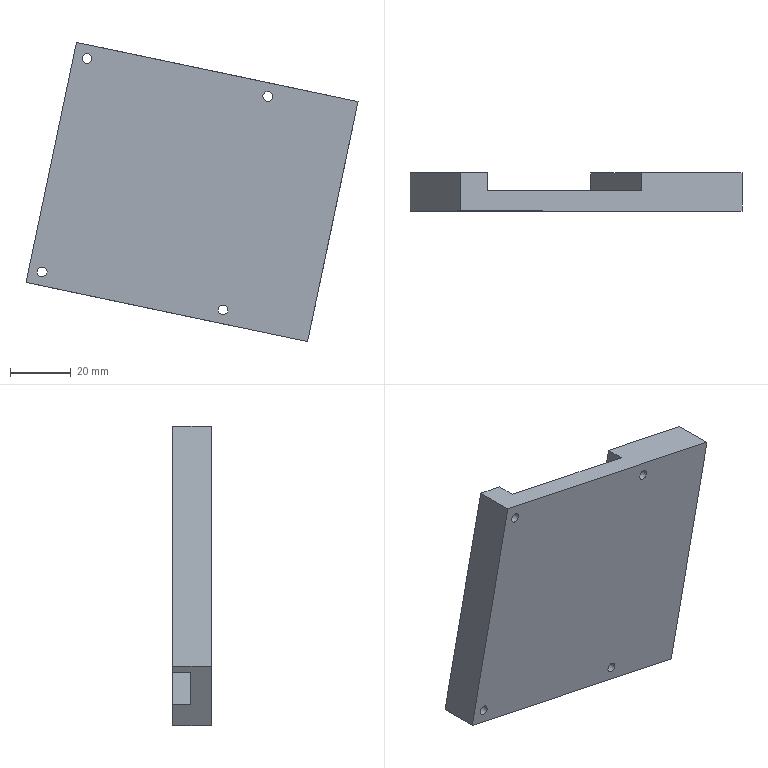Part | STEP file | 2_ESTAGIO_010 | 1 solid | 18 faces | box 109.627 x 12.7 x 98.805 mm | volume 71258 mm3 | plane 10 | cylinder 6 | cone 2 | commonest cylinder face diameters 3.242 x4 4.917 x2
STEP:
#1=CARTESIAN_POINT('',(0.,0.,0.));
#2=DIRECTION('',(0.,0.,1.));
#3=DIRECTION('',(1.,0.,0.));
#4=AXIS2_PLACEMENT_3D('',#1,#2,#3);
#5=CARTESIAN_POINT('',(428.339,-542.821,373.692));
#6=VERTEX_POINT('',#5);
#7=CARTESIAN_POINT('',(427.895,-544.,371.581));
#8=DIRECTION('',(0.9786,0.,-0.2056));
#9=DIRECTION('',(0.2056,0.,0.9786));
#10=AXIS2_PLACEMENT_3D('',#7,#8,#9);
#11=CIRCLE('',#10,2.458);
#12=CARTESIAN_POINT('',(427.071,-544.,371.754));
#13=DIRECTION('',(0.9786,0.,-0.2056));
#14=DIRECTION('',(0.1805,0.4794,0.8588));
#15=AXIS2_PLACEMENT_3D('',#12,#13,#14);
#16=CONICAL_SURFACE('',#15,1.,1.047);
#17=CARTESIAN_POINT('',(-5.783,0.8421));
#18=DIRECTION('',(1.,0.));
#19=VECTOR('',#18,1.);
#20=LINE('',#17,#19);
#21=(GEOMETRIC_REPRESENTATION_CONTEXT(2)PARAMETRIC_REPRESENTATION_CONTEXT()REPRESENTATION_CONTEXT('',''));
#22=DEFINITIONAL_REPRESENTATION('',(#20),#21);
#23=PCURVE('',#16,#22);
#24=CARTESIAN_POINT('',(447.37,-544.,367.488));
#25=DIRECTION('',(-0.9786,0.,0.2056));
#26=DIRECTION('',(0.1805,0.4794,0.8588));
#27=AXIS2_PLACEMENT_3D('',#24,#25,#26);
#28=CYLINDRICAL_SURFACE('',#27,2.458);
#29=CARTESIAN_POINT('',(12.066,19.9));
#30=DIRECTION('',(-1.,0.));
#31=VECTOR('',#30,1.);
#32=LINE('',#29,#31);
#33=(GEOMETRIC_REPRESENTATION_CONTEXT(2)PARAMETRIC_REPRESENTATION_CONTEXT()REPRESENTATION_CONTEXT('',''));
#34=DEFINITIONAL_REPRESENTATION('',(#32),#33);
#35=PCURVE('',#28,#34);
#36=SURFACE_CURVE('',#11,(#23,#35),.PCURVE_S1.);
#37=EDGE_CURVE('',#6,#6,#36,.T.);
#38=ORIENTED_EDGE('',*,*,#37,.F.);
#39=CARTESIAN_POINT('',(426.506,-544.,371.873));
#40=VERTEX_POINT('',#39);
#41=CARTESIAN_POINT('',(426.506,-544.,371.873));
#42=CARTESIAN_POINT('',(428.339,-542.821,373.692));
#43=B_SPLINE_CURVE_WITH_KNOTS('',1,(#41,#42),.UNSPECIFIED.,.F.,.F.,(2,2),(-1.155,1.684),.PIECEWISE_BEZIER_KNOTS.);
#44=CARTESIAN_POINT('',(0.,0.));
#45=DIRECTION('',(0.,1.));
#46=VECTOR('',#45,1.);
#47=LINE('',#44,#46);
#48=(GEOMETRIC_REPRESENTATION_CONTEXT(2)PARAMETRIC_REPRESENTATION_CONTEXT()REPRESENTATION_CONTEXT('',''));
#49=DEFINITIONAL_REPRESENTATION('',(#47),#48);
#50=PCURVE('',#16,#49);
#51=CARTESIAN_POINT('',(6.283,0.));
#52=DIRECTION('',(0.,1.));
#53=VECTOR('',#52,1.);
#54=LINE('',#51,#53);
#55=(GEOMETRIC_REPRESENTATION_CONTEXT(2)PARAMETRIC_REPRESENTATION_CONTEXT()REPRESENTATION_CONTEXT('',''));
#56=DEFINITIONAL_REPRESENTATION('',(#54),#55);
#57=PCURVE('',#16,#56);
#58=SEAM_CURVE('',#43,(#50,#57),.PCURVE_S1.);
#59=EDGE_CURVE('',#40,#6,#58,.T.);
#60=ORIENTED_EDGE('',*,*,#59,.F.);
#61=ORIENTED_EDGE('',*,*,#59,.T.);
#62=EDGE_LOOP('',(#38,#60,#61));
#63=FACE_BOUND('',#62,.F.);
#64=ADVANCED_FACE('',(#63),#16,.F.);
#65=CARTESIAN_POINT('',(443.355,-537.65,347.895));
#66=VERTEX_POINT('',#65);
#67=CARTESIAN_POINT('',(460.012,-537.65,427.164));
#68=VERTEX_POINT('',#67);
#69=CARTESIAN_POINT('',(443.355,-537.65,347.895));
#70=DIRECTION('',(0.2056,0.,0.9786));
#71=VECTOR('',#70,1.);
#72=LINE('',#69,#71);
#73=CARTESIAN_POINT('',(442.944,-550.35,345.938));
#74=DIRECTION('',(0.9786,0.,-0.2056));
#75=DIRECTION('',(-0.2056,0.,-0.9786));
#76=AXIS2_PLACEMENT_3D('',#73,#74,#75);
#77=PLANE('',#76);
#78=CARTESIAN_POINT('',(-2.,12.7));
#79=DIRECTION('',(-1.,0.));
#80=VECTOR('',#79,1.);
#81=LINE('',#78,#80);
#82=(GEOMETRIC_REPRESENTATION_CONTEXT(2)PARAMETRIC_REPRESENTATION_CONTEXT()REPRESENTATION_CONTEXT('',''));
#83=DEFINITIONAL_REPRESENTATION('',(#81),#82);
#84=PCURVE('',#77,#83);
#85=CARTESIAN_POINT('',(413.585,-537.65,352.107));
#86=DIRECTION('',(0.,1.,0.));
#87=DIRECTION('',(0.,0.,1.));
#88=AXIS2_PLACEMENT_3D('',#85,#86,#87);
#89=PLANE('',#88);
#90=CARTESIAN_POINT('',(-4.212,29.77));
#91=DIRECTION('',(0.9786,0.2056));
#92=VECTOR('',#91,1.);
#93=LINE('',#90,#92);
#94=(GEOMETRIC_REPRESENTATION_CONTEXT(2)PARAMETRIC_REPRESENTATION_CONTEXT()REPRESENTATION_CONTEXT('',''));
#95=DEFINITIONAL_REPRESENTATION('',(#93),#94);
#96=PCURVE('',#89,#95);
#97=SURFACE_CURVE('',#72,(#84,#96),.PCURVE_S1.);
#98=EDGE_CURVE('',#66,#68,#97,.T.);
#99=ORIENTED_EDGE('',*,*,#98,.T.);
#100=CARTESIAN_POINT('',(460.012,-550.35,427.164));
#101=VERTEX_POINT('',#100);
#102=CARTESIAN_POINT('',(460.012,-550.35,427.164));
#103=DIRECTION('',(0.,1.,0.));
#104=VECTOR('',#103,1.);
#105=LINE('',#102,#104);
#106=CARTESIAN_POINT('',(-83.,0.));
#107=DIRECTION('',(0.,1.));
#108=VECTOR('',#107,1.);
#109=LINE('',#106,#108);
#110=(GEOMETRIC_REPRESENTATION_CONTEXT(2)PARAMETRIC_REPRESENTATION_CONTEXT()REPRESENTATION_CONTEXT('',''));
#111=DEFINITIONAL_REPRESENTATION('',(#109),#110);
#112=PCURVE('',#77,#111);
#113=CARTESIAN_POINT('',(105.419,0.,501.676));
#114=DIRECTION('',(0.2056,0.,0.9786));
#115=DIRECTION('',(0.9786,0.,-0.2056));
#116=AXIS2_PLACEMENT_3D('',#113,#114,#115);
#117=PLANE('',#116);
#118=CARTESIAN_POINT('',(362.337,-550.35));
#119=DIRECTION('',(0.,1.));
#120=VECTOR('',#119,1.);
#121=LINE('',#118,#120);
#122=(GEOMETRIC_REPRESENTATION_CONTEXT(2)PARAMETRIC_REPRESENTATION_CONTEXT()REPRESENTATION_CONTEXT('',''));
#123=DEFINITIONAL_REPRESENTATION('',(#121),#122);
#124=PCURVE('',#117,#123);
#125=SURFACE_CURVE('',#105,(#112,#124),.PCURVE_S1.);
#126=EDGE_CURVE('',#101,#68,#125,.T.);
#127=ORIENTED_EDGE('',*,*,#126,.F.);
#128=CARTESIAN_POINT('',(443.355,-550.35,347.895));
#129=VERTEX_POINT('',#128);
#130=CARTESIAN_POINT('',(443.355,-550.35,347.895));
#131=DIRECTION('',(0.2056,0.,0.9786));
#132=VECTOR('',#131,1.);
#133=LINE('',#130,#132);
#134=CARTESIAN_POINT('',(-2.,0.));
#135=DIRECTION('',(-1.,0.));
#136=VECTOR('',#135,1.);
#137=LINE('',#134,#136);
#138=(GEOMETRIC_REPRESENTATION_CONTEXT(2)PARAMETRIC_REPRESENTATION_CONTEXT()REPRESENTATION_CONTEXT('',''));
#139=DEFINITIONAL_REPRESENTATION('',(#137),#138);
#140=PCURVE('',#77,#139);
#141=CARTESIAN_POINT('',(354.867,-550.35,364.446));
#142=DIRECTION('',(0.,-1.,0.));
#143=DIRECTION('',(0.,0.,-1.));
#144=AXIS2_PLACEMENT_3D('',#141,#142,#143);
#145=PLANE('',#144);
#146=CARTESIAN_POINT('',(16.551,88.488));
#147=DIRECTION('',(-0.9786,0.2056));
#148=VECTOR('',#147,1.);
#149=LINE('',#146,#148);
#150=(GEOMETRIC_REPRESENTATION_CONTEXT(2)PARAMETRIC_REPRESENTATION_CONTEXT()REPRESENTATION_CONTEXT('',''));
#151=DEFINITIONAL_REPRESENTATION('',(#149),#150);
#152=PCURVE('',#145,#151);
#153=SURFACE_CURVE('',#133,(#140,#152),.PCURVE_S1.);
#154=EDGE_CURVE('',#129,#101,#153,.T.);
#155=ORIENTED_EDGE('',*,*,#154,.F.);
#156=CARTESIAN_POINT('',(443.355,-550.35,347.895));
#157=DIRECTION('',(0.,1.,0.));
#158=VECTOR('',#157,1.);
#159=LINE('',#156,#158);
#160=CARTESIAN_POINT('',(-2.,0.));
#161=DIRECTION('',(0.,1.));
#162=VECTOR('',#161,1.);
#163=LINE('',#160,#162);
#164=(GEOMETRIC_REPRESENTATION_CONTEXT(2)PARAMETRIC_REPRESENTATION_CONTEXT()REPRESENTATION_CONTEXT('',''));
#165=DEFINITIONAL_REPRESENTATION('',(#163),#164);
#166=PCURVE('',#77,#165);
#167=CARTESIAN_POINT('',(88.762,0.,422.407));
#168=DIRECTION('',(0.2056,0.,0.9786));
#169=DIRECTION('',(0.9786,0.,-0.2056));
#170=AXIS2_PLACEMENT_3D('',#167,#168,#169);
#171=PLANE('',#170);
#172=CARTESIAN_POINT('',(362.337,-550.35));
#173=DIRECTION('',(0.,1.));
#174=VECTOR('',#173,1.);
#175=LINE('',#172,#174);
#176=(GEOMETRIC_REPRESENTATION_CONTEXT(2)PARAMETRIC_REPRESENTATION_CONTEXT()REPRESENTATION_CONTEXT('',''));
#177=DEFINITIONAL_REPRESENTATION('',(#175),#176);
#178=PCURVE('',#171,#177);
#179=SURFACE_CURVE('',#159,(#166,#178),.PCURVE_S1.);
#180=EDGE_CURVE('',#129,#66,#179,.T.);
#181=ORIENTED_EDGE('',*,*,#180,.T.);
#182=EDGE_LOOP('',(#99,#127,#155,#181));
#183=FACE_BOUND('',#182,.T.);
#184=CARTESIAN_POINT('',(447.912,-542.821,369.579));
#185=VERTEX_POINT('',#184);
#186=CARTESIAN_POINT('',(447.468,-544.,367.468));
#187=DIRECTION('',(0.9786,0.,-0.2056));
#188=DIRECTION('',(0.1805,0.4794,0.8588));
#189=AXIS2_PLACEMENT_3D('',#186,#187,#188);
#190=CIRCLE('',#189,2.458);
#191=CARTESIAN_POINT('',(-22.,6.35));
#192=DIRECTION('',(-0.8776,0.4794));
#193=AXIS2_PLACEMENT_2D('',#191,#192);
#194=CIRCLE('',#193,2.458);
#195=(GEOMETRIC_REPRESENTATION_CONTEXT(2)PARAMETRIC_REPRESENTATION_CONTEXT()REPRESENTATION_CONTEXT('',''));
#196=DEFINITIONAL_REPRESENTATION('',(#194),#195);
#197=PCURVE('',#77,#196);
#198=CARTESIAN_POINT('',(6.283,-0.1));
#199=DIRECTION('',(-1.,0.));
#200=VECTOR('',#199,1.);
#201=LINE('',#198,#200);
#202=(GEOMETRIC_REPRESENTATION_CONTEXT(2)PARAMETRIC_REPRESENTATION_CONTEXT()REPRESENTATION_CONTEXT('',''));
#203=DEFINITIONAL_REPRESENTATION('',(#201),#202);
#204=PCURVE('',#28,#203);
#205=SURFACE_CURVE('',#190,(#197,#204),.PCURVE_S1.);
#206=EDGE_CURVE('',#185,#185,#205,.T.);
#207=ORIENTED_EDGE('',*,*,#206,.F.);
#208=EDGE_LOOP('',(#207));
#209=FACE_BOUND('',#208,.T.);
#210=CARTESIAN_POINT('',(456.343,-542.821,409.703));
#211=VERTEX_POINT('',#210);
#212=CARTESIAN_POINT('',(455.899,-544.,407.592));
#213=DIRECTION('',(0.9786,0.,-0.2056));
#214=DIRECTION('',(0.1805,0.4794,0.8588));
#215=AXIS2_PLACEMENT_3D('',#212,#213,#214);
#216=CIRCLE('',#215,2.458);
#217=CARTESIAN_POINT('',(-63.,6.35));
#218=DIRECTION('',(-0.8776,0.4794));
#219=AXIS2_PLACEMENT_2D('',#217,#218);
#220=CIRCLE('',#219,2.458);
#221=(GEOMETRIC_REPRESENTATION_CONTEXT(2)PARAMETRIC_REPRESENTATION_CONTEXT()REPRESENTATION_CONTEXT('',''));
#222=DEFINITIONAL_REPRESENTATION('',(#220),#221);
#223=PCURVE('',#77,#222);
#224=CARTESIAN_POINT('',(455.801,-544.,407.612));
#225=DIRECTION('',(-0.9786,0.,0.2056));
#226=DIRECTION('',(0.1805,0.4794,0.8588));
#227=AXIS2_PLACEMENT_3D('',#224,#225,#226);
#228=CYLINDRICAL_SURFACE('',#227,2.458);
#229=CARTESIAN_POINT('',(6.283,-0.1));
#230=DIRECTION('',(-1.,0.));
#231=VECTOR('',#230,1.);
#232=LINE('',#229,#231);
#233=(GEOMETRIC_REPRESENTATION_CONTEXT(2)PARAMETRIC_REPRESENTATION_CONTEXT()REPRESENTATION_CONTEXT('',''));
#234=DEFINITIONAL_REPRESENTATION('',(#232),#233);
#235=PCURVE('',#228,#234);
#236=SURFACE_CURVE('',#216,(#223,#235),.PCURVE_S1.);
#237=EDGE_CURVE('',#211,#211,#236,.T.);
#238=ORIENTED_EDGE('',*,*,#237,.F.);
#239=EDGE_LOOP('',(#238));
#240=FACE_BOUND('',#239,.T.);
#241=ADVANCED_FACE('',(#183,#209,#240),#77,.T.);
#242=CARTESIAN_POINT('',(410.082,-537.65,354.887));
#243=VERTEX_POINT('',#242);
#244=CARTESIAN_POINT('',(410.082,-537.65,354.887));
#245=DIRECTION('',(0.9786,0.,-0.2056));
#246=VECTOR('',#245,1.);
#247=LINE('',#244,#246);
#248=CARTESIAN_POINT('',(2.78,-3.503));
#249=DIRECTION('',(-0.2056,0.9786));
#250=VECTOR('',#249,1.);
#251=LINE('',#248,#250);
#252=(GEOMETRIC_REPRESENTATION_CONTEXT(2)PARAMETRIC_REPRESENTATION_CONTEXT()REPRESENTATION_CONTEXT('',''));
#253=DEFINITIONAL_REPRESENTATION('',(#251),#252);
#254=PCURVE('',#89,#253);
#255=CARTESIAN_POINT('',(328.337,-537.65));
#256=DIRECTION('',(1.,0.));
#257=VECTOR('',#256,1.);
#258=LINE('',#255,#257);
#259=(GEOMETRIC_REPRESENTATION_CONTEXT(2)PARAMETRIC_REPRESENTATION_CONTEXT()REPRESENTATION_CONTEXT('',''));
#260=DEFINITIONAL_REPRESENTATION('',(#258),#259);
#261=PCURVE('',#171,#260);
#262=SURFACE_CURVE('',#247,(#254,#261),.PCURVE_S1.);
#263=EDGE_CURVE('',#243,#66,#262,.T.);
#264=ORIENTED_EDGE('',*,*,#263,.F.);
#265=CARTESIAN_POINT('',(426.739,-537.65,434.156));
#266=VERTEX_POINT('',#265);
#267=CARTESIAN_POINT('',(410.082,-537.65,354.887));
#268=DIRECTION('',(0.2056,0.,0.9786));
#269=VECTOR('',#268,1.);
#270=LINE('',#267,#269);
#271=CARTESIAN_POINT('',(2.78,-3.503));
#272=DIRECTION('',(0.9786,0.2056));
#273=VECTOR('',#272,1.);
#274=LINE('',#271,#273);
#275=(GEOMETRIC_REPRESENTATION_CONTEXT(2)PARAMETRIC_REPRESENTATION_CONTEXT()REPRESENTATION_CONTEXT('',''));
#276=DEFINITIONAL_REPRESENTATION('',(#274),#275);
#277=PCURVE('',#89,#276);
#278=CARTESIAN_POINT('',(409.67,-537.65,352.93));
#279=DIRECTION('',(-0.9786,0.,0.2056));
#280=DIRECTION('',(0.2056,0.,0.9786));
#281=AXIS2_PLACEMENT_3D('',#278,#279,#280);
#282=PLANE('',#281);
#283=CARTESIAN_POINT('',(2.,0.));
#284=DIRECTION('',(1.,0.));
#285=VECTOR('',#284,1.);
#286=LINE('',#283,#285);
#287=(GEOMETRIC_REPRESENTATION_CONTEXT(2)PARAMETRIC_REPRESENTATION_CONTEXT()REPRESENTATION_CONTEXT('',''));
#288=DEFINITIONAL_REPRESENTATION('',(#286),#287);
#289=PCURVE('',#282,#288);
#290=SURFACE_CURVE('',#270,(#277,#289),.PCURVE_S1.);
#291=EDGE_CURVE('',#243,#266,#290,.T.);
#292=ORIENTED_EDGE('',*,*,#291,.T.);
#293=CARTESIAN_POINT('',(426.739,-537.65,434.156));
#294=DIRECTION('',(0.9786,0.,-0.2056));
#295=VECTOR('',#294,1.);
#296=LINE('',#293,#295);
#297=CARTESIAN_POINT('',(82.049,13.154));
#298=DIRECTION('',(-0.2056,0.9786));
#299=VECTOR('',#298,1.);
#300=LINE('',#297,#299);
#301=(GEOMETRIC_REPRESENTATION_CONTEXT(2)PARAMETRIC_REPRESENTATION_CONTEXT()REPRESENTATION_CONTEXT('',''));
#302=DEFINITIONAL_REPRESENTATION('',(#300),#301);
#303=PCURVE('',#89,#302);
#304=CARTESIAN_POINT('',(328.337,-537.65));
#305=DIRECTION('',(1.,0.));
#306=VECTOR('',#305,1.);
#307=LINE('',#304,#306);
#308=(GEOMETRIC_REPRESENTATION_CONTEXT(2)PARAMETRIC_REPRESENTATION_CONTEXT()REPRESENTATION_CONTEXT('',''));
#309=DEFINITIONAL_REPRESENTATION('',(#307),#308);
#310=PCURVE('',#117,#309);
#311=SURFACE_CURVE('',#296,(#303,#310),.PCURVE_S1.);
#312=EDGE_CURVE('',#266,#68,#311,.T.);
#313=ORIENTED_EDGE('',*,*,#312,.T.);
#314=ORIENTED_EDGE('',*,*,#98,.F.);
#315=EDGE_LOOP('',(#264,#292,#313,#314));
#316=FACE_BOUND('',#315,.T.);
#317=CARTESIAN_POINT('',(428.795,-537.65,428.05));
#318=VERTEX_POINT('',#317);
#319=CARTESIAN_POINT('',(430.217,-537.65,428.827));
#320=DIRECTION('',(0.,1.,0.));
#321=DIRECTION('',(1.,0.,0.));
#322=AXIS2_PLACEMENT_3D('',#319,#320,#321);
#323=CIRCLE('',#322,1.621);
#324=CARTESIAN_POINT('',(76.719,16.632));
#325=DIRECTION('',(0.,1.));
#326=AXIS2_PLACEMENT_2D('',#324,#325);
#327=CIRCLE('',#326,1.621);
#328=(GEOMETRIC_REPRESENTATION_CONTEXT(2)PARAMETRIC_REPRESENTATION_CONTEXT()REPRESENTATION_CONTEXT('',''));
#329=DEFINITIONAL_REPRESENTATION('',(#327),#328);
#330=PCURVE('',#89,#329);
#331=CARTESIAN_POINT('',(430.217,-537.75,428.827));
#332=DIRECTION('',(0.,-1.,0.));
#333=DIRECTION('',(0.8776,0.,0.4794));
#334=AXIS2_PLACEMENT_3D('',#331,#332,#333);
#335=CYLINDRICAL_SURFACE('',#334,1.621);
#336=CARTESIAN_POINT('',(12.066,-0.1));
#337=DIRECTION('',(-1.,0.));
#338=VECTOR('',#337,1.);
#339=LINE('',#336,#338);
#340=(GEOMETRIC_REPRESENTATION_CONTEXT(2)PARAMETRIC_REPRESENTATION_CONTEXT()REPRESENTATION_CONTEXT('',''));
#341=DEFINITIONAL_REPRESENTATION('',(#339),#340);
#342=PCURVE('',#335,#341);
#343=SURFACE_CURVE('',#323,(#330,#342),.PCURVE_S1.);
#344=EDGE_CURVE('',#318,#318,#343,.T.);
#345=ORIENTED_EDGE('',*,*,#344,.F.);
#346=EDGE_LOOP('',(#345));
#347=FACE_BOUND('',#346,.T.);
#348=CARTESIAN_POINT('',(413.988,-537.65,357.588));
#349=VERTEX_POINT('',#348);
#350=CARTESIAN_POINT('',(415.411,-537.65,358.366));
#351=DIRECTION('',(0.,1.,0.));
#352=DIRECTION('',(1.,0.,0.));
#353=AXIS2_PLACEMENT_3D('',#350,#351,#352);
#354=CIRCLE('',#353,1.621);
#355=CARTESIAN_POINT('',(6.258,1.826));
#356=DIRECTION('',(0.,1.));
#357=AXIS2_PLACEMENT_2D('',#355,#356);
#358=CIRCLE('',#357,1.621);
#359=(GEOMETRIC_REPRESENTATION_CONTEXT(2)PARAMETRIC_REPRESENTATION_CONTEXT()REPRESENTATION_CONTEXT('',''));
#360=DEFINITIONAL_REPRESENTATION('',(#358),#359);
#361=PCURVE('',#89,#360);
#362=CARTESIAN_POINT('',(415.411,-537.75,358.366));
#363=DIRECTION('',(0.,-1.,0.));
#364=DIRECTION('',(0.8776,0.,0.4794));
#365=AXIS2_PLACEMENT_3D('',#362,#363,#364);
#366=CYLINDRICAL_SURFACE('',#365,1.621);
#367=CARTESIAN_POINT('',(12.066,-0.1));
#368=DIRECTION('',(-1.,0.));
#369=VECTOR('',#368,1.);
#370=LINE('',#367,#369);
#371=(GEOMETRIC_REPRESENTATION_CONTEXT(2)PARAMETRIC_REPRESENTATION_CONTEXT()REPRESENTATION_CONTEXT('',''));
#372=DEFINITIONAL_REPRESENTATION('',(#370),#371);
#373=PCURVE('',#366,#372);
#374=SURFACE_CURVE('',#354,(#361,#373),.PCURVE_S1.);
#375=EDGE_CURVE('',#349,#349,#374,.T.);
#376=ORIENTED_EDGE('',*,*,#375,.F.);
#377=EDGE_LOOP('',(#376));
#378=FACE_BOUND('',#377,.T.);
#379=ADVANCED_FACE('',(#316,#347,#378),#89,.T.);
#380=CARTESIAN_POINT('',(350.385,-550.35,367.431));
#381=VERTEX_POINT('',#380);
#382=CARTESIAN_POINT('',(350.385,-550.35,367.431));
#383=DIRECTION('',(0.9786,0.,-0.2056));
#384=VECTOR('',#383,1.);
#385=LINE('',#382,#384);
#386=CARTESIAN_POINT('',(267.337,-550.35));
#387=DIRECTION('',(1.,0.));
#388=VECTOR('',#387,1.);
#389=LINE('',#386,#388);
#390=(GEOMETRIC_REPRESENTATION_CONTEXT(2)PARAMETRIC_REPRESENTATION_CONTEXT()REPRESENTATION_CONTEXT('',''));
#391=DEFINITIONAL_REPRESENTATION('',(#389),#390);
#392=PCURVE('',#171,#391);
#393=CARTESIAN_POINT('',(-2.985,-4.482));
#394=DIRECTION('',(0.2056,0.9786));
#395=VECTOR('',#394,1.);
#396=LINE('',#393,#395);
#397=(GEOMETRIC_REPRESENTATION_CONTEXT(2)PARAMETRIC_REPRESENTATION_CONTEXT()REPRESENTATION_CONTEXT('',''));
#398=DEFINITIONAL_REPRESENTATION('',(#396),#397);
#399=PCURVE('',#145,#398);
#400=SURFACE_CURVE('',#385,(#392,#399),.PCURVE_S1.);
#401=EDGE_CURVE('',#381,#129,#400,.T.);
#402=ORIENTED_EDGE('',*,*,#401,.F.);
#403=CARTESIAN_POINT('',(350.385,-537.65,367.431));
#404=VERTEX_POINT('',#403);
#405=CARTESIAN_POINT('',(350.385,-537.65,367.431));
#406=DIRECTION('',(0.,-1.,0.));
#407=VECTOR('',#406,1.);
#408=LINE('',#405,#407);
#409=CARTESIAN_POINT('',(267.337,-537.65));
#410=DIRECTION('',(0.,-1.));
#411=VECTOR('',#410,1.);
#412=LINE('',#409,#411);
#413=(GEOMETRIC_REPRESENTATION_CONTEXT(2)PARAMETRIC_REPRESENTATION_CONTEXT()REPRESENTATION_CONTEXT('',''));
#414=DEFINITIONAL_REPRESENTATION('',(#412),#413);
#415=PCURVE('',#171,#414);
#416=CARTESIAN_POINT('',(349.974,-537.65,365.474));
#417=DIRECTION('',(-0.9786,0.,0.2056));
#418=DIRECTION('',(0.2056,0.,0.9786));
#419=AXIS2_PLACEMENT_3D('',#416,#417,#418);
#420=PLANE('',#419);
#421=CARTESIAN_POINT('',(2.,0.));
#422=DIRECTION('',(0.,-1.));
#423=VECTOR('',#422,1.);
#424=LINE('',#421,#423);
#425=(GEOMETRIC_REPRESENTATION_CONTEXT(2)PARAMETRIC_REPRESENTATION_CONTEXT()REPRESENTATION_CONTEXT('',''));
#426=DEFINITIONAL_REPRESENTATION('',(#424),#425);
#427=PCURVE('',#420,#426);
#428=SURFACE_CURVE('',#408,(#415,#427),.PCURVE_S1.);
#429=EDGE_CURVE('',#404,#381,#428,.T.);
#430=ORIENTED_EDGE('',*,*,#429,.F.);
#431=CARTESIAN_POINT('',(359.193,-537.65,365.581));
#432=VERTEX_POINT('',#431);
#433=CARTESIAN_POINT('',(350.385,-537.65,367.431));
#434=DIRECTION('',(0.9786,0.,-0.2056));
#435=VECTOR('',#434,1.);
#436=LINE('',#433,#435);
#437=CARTESIAN_POINT('',(267.337,-537.65));
#438=DIRECTION('',(1.,0.));
#439=VECTOR('',#438,1.);
#440=LINE('',#437,#439);
#441=(GEOMETRIC_REPRESENTATION_CONTEXT(2)PARAMETRIC_REPRESENTATION_CONTEXT()REPRESENTATION_CONTEXT('',''));
#442=DEFINITIONAL_REPRESENTATION('',(#440),#441);
#443=PCURVE('',#171,#442);
#444=CARTESIAN_POINT('',(413.585,-537.65,352.107));
#445=DIRECTION('',(0.,1.,0.));
#446=DIRECTION('',(0.,0.,1.));
#447=AXIS2_PLACEMENT_3D('',#444,#445,#446);
#448=PLANE('',#447);
#449=CARTESIAN_POINT('',(15.324,-63.199));
#450=DIRECTION('',(-0.2056,0.9786));
#451=VECTOR('',#450,1.);
#452=LINE('',#449,#451);
#453=(GEOMETRIC_REPRESENTATION_CONTEXT(2)PARAMETRIC_REPRESENTATION_CONTEXT()REPRESENTATION_CONTEXT('',''));
#454=DEFINITIONAL_REPRESENTATION('',(#452),#453);
#455=PCURVE('',#448,#454);
#456=SURFACE_CURVE('',#436,(#443,#455),.PCURVE_S1.);
#457=EDGE_CURVE('',#404,#432,#456,.T.);
#458=ORIENTED_EDGE('',*,*,#457,.T.);
#459=CARTESIAN_POINT('',(359.193,-543.65,365.581));
#460=VERTEX_POINT('',#459);
#461=CARTESIAN_POINT('',(359.193,-543.65,365.581));
#462=DIRECTION('',(0.,1.,0.));
#463=VECTOR('',#462,1.);
#464=LINE('',#461,#463);
#465=CARTESIAN_POINT('',(276.337,-543.65));
#466=DIRECTION('',(0.,1.));
#467=VECTOR('',#466,1.);
#468=LINE('',#465,#467);
#469=(GEOMETRIC_REPRESENTATION_CONTEXT(2)PARAMETRIC_REPRESENTATION_CONTEXT()REPRESENTATION_CONTEXT('',''));
#470=DEFINITIONAL_REPRESENTATION('',(#468),#469);
#471=PCURVE('',#171,#470);
#472=CARTESIAN_POINT('',(358.782,-543.65,363.623));
#473=DIRECTION('',(0.9786,0.,-0.2056));
#474=DIRECTION('',(-0.2056,0.,-0.9786));
#475=AXIS2_PLACEMENT_3D('',#472,#473,#474);
#476=PLANE('',#475);
#477=CARTESIAN_POINT('',(-2.,0.));
#478=DIRECTION('',(0.,1.));
#479=VECTOR('',#478,1.);
#480=LINE('',#477,#479);
#481=(GEOMETRIC_REPRESENTATION_CONTEXT(2)PARAMETRIC_REPRESENTATION_CONTEXT()REPRESENTATION_CONTEXT('',''));
#482=DEFINITIONAL_REPRESENTATION('',(#480),#481);
#483=PCURVE('',#476,#482);
#484=SURFACE_CURVE('',#464,(#471,#483),.PCURVE_S1.);
#485=EDGE_CURVE('',#460,#432,#484,.T.);
#486=ORIENTED_EDGE('',*,*,#485,.F.);
#487=CARTESIAN_POINT('',(410.082,-543.65,354.887));
#488=VERTEX_POINT('',#487);
#489=CARTESIAN_POINT('',(410.082,-543.65,354.887));
#490=DIRECTION('',(-0.9786,0.,0.2056));
#491=VECTOR('',#490,1.);
#492=LINE('',#489,#491);
#493=CARTESIAN_POINT('',(328.337,-543.65));
#494=DIRECTION('',(-1.,0.));
#495=VECTOR('',#494,1.);
#496=LINE('',#493,#495);
#497=(GEOMETRIC_REPRESENTATION_CONTEXT(2)PARAMETRIC_REPRESENTATION_CONTEXT()REPRESENTATION_CONTEXT('',''));
#498=DEFINITIONAL_REPRESENTATION('',(#496),#497);
#499=PCURVE('',#171,#498);
#500=CARTESIAN_POINT('',(409.67,-543.65,352.93));
#501=DIRECTION('',(0.,1.,0.));
#502=DIRECTION('',(0.,0.,1.));
#503=AXIS2_PLACEMENT_3D('',#500,#501,#502);
#504=PLANE('',#503);
#505=CARTESIAN_POINT('',(1.957,0.4113));
#506=DIRECTION('',(0.2056,-0.9786));
#507=VECTOR('',#506,1.);
#508=LINE('',#505,#507);
#509=(GEOMETRIC_REPRESENTATION_CONTEXT(2)PARAMETRIC_REPRESENTATION_CONTEXT()REPRESENTATION_CONTEXT('',''));
#510=DEFINITIONAL_REPRESENTATION('',(#508),#509);
#511=PCURVE('',#504,#510);
#512=SURFACE_CURVE('',#492,(#499,#511),.PCURVE_S1.);
#513=EDGE_CURVE('',#488,#460,#512,.T.);
#514=ORIENTED_EDGE('',*,*,#513,.F.);
#515=CARTESIAN_POINT('',(410.082,-537.65,354.887));
#516=DIRECTION('',(0.,-1.,0.));
#517=VECTOR('',#516,1.);
#518=LINE('',#515,#517);
#519=CARTESIAN_POINT('',(328.337,-537.65));
#520=DIRECTION('',(0.,-1.));
#521=VECTOR('',#520,1.);
#522=LINE('',#519,#521);
#523=(GEOMETRIC_REPRESENTATION_CONTEXT(2)PARAMETRIC_REPRESENTATION_CONTEXT()REPRESENTATION_CONTEXT('',''));
#524=DEFINITIONAL_REPRESENTATION('',(#522),#523);
#525=PCURVE('',#171,#524);
#526=CARTESIAN_POINT('',(2.,0.));
#527=DIRECTION('',(0.,-1.));
#528=VECTOR('',#527,1.);
#529=LINE('',#526,#528);
#530=(GEOMETRIC_REPRESENTATION_CONTEXT(2)PARAMETRIC_REPRESENTATION_CONTEXT()REPRESENTATION_CONTEXT('',''));
#531=DEFINITIONAL_REPRESENTATION('',(#529),#530);
#532=PCURVE('',#282,#531);
#533=SURFACE_CURVE('',#518,(#525,#532),.PCURVE_S1.);
#534=EDGE_CURVE('',#243,#488,#533,.T.);
#535=ORIENTED_EDGE('',*,*,#534,.F.);
#536=ORIENTED_EDGE('',*,*,#263,.T.);
#537=ORIENTED_EDGE('',*,*,#180,.F.);
#538=EDGE_LOOP('',(#402,#430,#458,#486,#514,#535,#536,#537));
#539=FACE_BOUND('',#538,.T.);
#540=ADVANCED_FACE('',(#539),#171,.F.);
#541=ORIENTED_EDGE('',*,*,#291,.F.);
#542=ORIENTED_EDGE('',*,*,#534,.T.);
#543=CARTESIAN_POINT('',(426.739,-543.65,434.156));
#544=VERTEX_POINT('',#543);
#545=CARTESIAN_POINT('',(410.082,-543.65,354.887));
#546=DIRECTION('',(0.2056,0.,0.9786));
#547=VECTOR('',#546,1.);
#548=LINE('',#545,#547);
#549=CARTESIAN_POINT('',(2.,-6.));
#550=DIRECTION('',(1.,0.));
#551=VECTOR('',#550,1.);
#552=LINE('',#549,#551);
#553=(GEOMETRIC_REPRESENTATION_CONTEXT(2)PARAMETRIC_REPRESENTATION_CONTEXT()REPRESENTATION_CONTEXT('',''));
#554=DEFINITIONAL_REPRESENTATION('',(#552),#553);
#555=PCURVE('',#282,#554);
#556=CARTESIAN_POINT('',(1.957,0.4113));
#557=DIRECTION('',(0.9786,0.2056));
#558=VECTOR('',#557,1.);
#559=LINE('',#556,#558);
#560=(GEOMETRIC_REPRESENTATION_CONTEXT(2)PARAMETRIC_REPRESENTATION_CONTEXT()REPRESENTATION_CONTEXT('',''));
#561=DEFINITIONAL_REPRESENTATION('',(#559),#560);
#562=PCURVE('',#504,#561);
#563=SURFACE_CURVE('',#548,(#555,#562),.PCURVE_S1.);
#564=EDGE_CURVE('',#488,#544,#563,.T.);
#565=ORIENTED_EDGE('',*,*,#564,.T.);
#566=CARTESIAN_POINT('',(426.739,-537.65,434.156));
#567=DIRECTION('',(0.,-1.,0.));
#568=VECTOR('',#567,1.);
#569=LINE('',#566,#568);
#570=CARTESIAN_POINT('',(83.,0.));
#571=DIRECTION('',(0.,-1.));
#572=VECTOR('',#571,1.);
#573=LINE('',#570,#572);
#574=(GEOMETRIC_REPRESENTATION_CONTEXT(2)PARAMETRIC_REPRESENTATION_CONTEXT()REPRESENTATION_CONTEXT('',''));
#575=DEFINITIONAL_REPRESENTATION('',(#573),#574);
#576=PCURVE('',#282,#575);
#577=CARTESIAN_POINT('',(328.337,-537.65));
#578=DIRECTION('',(0.,-1.));
#579=VECTOR('',#578,1.);
#580=LINE('',#577,#579);
#581=(GEOMETRIC_REPRESENTATION_CONTEXT(2)PARAMETRIC_REPRESENTATION_CONTEXT()REPRESENTATION_CONTEXT('',''));
#582=DEFINITIONAL_REPRESENTATION('',(#580),#581);
#583=PCURVE('',#117,#582);
#584=SURFACE_CURVE('',#569,(#576,#583),.PCURVE_S1.);
#585=EDGE_CURVE('',#266,#544,#584,.T.);
#586=ORIENTED_EDGE('',*,*,#585,.F.);
#587=EDGE_LOOP('',(#541,#542,#565,#586));
#588=FACE_BOUND('',#587,.T.);
#589=ADVANCED_FACE('',(#588),#282,.T.);
#590=ORIENTED_EDGE('',*,*,#457,.F.);
#591=CARTESIAN_POINT('',(367.043,-537.65,446.7));
#592=VERTEX_POINT('',#591);
#593=CARTESIAN_POINT('',(350.385,-537.65,367.431));
#594=DIRECTION('',(0.2056,0.,0.9786));
#595=VECTOR('',#594,1.);
#596=LINE('',#593,#595);
#597=CARTESIAN_POINT('',(15.324,-63.199));
#598=DIRECTION('',(0.9786,0.2056));
#599=VECTOR('',#598,1.);
#600=LINE('',#597,#599);
#601=(GEOMETRIC_REPRESENTATION_CONTEXT(2)PARAMETRIC_REPRESENTATION_CONTEXT()REPRESENTATION_CONTEXT('',''));
#602=DEFINITIONAL_REPRESENTATION('',(#600),#601);
#603=PCURVE('',#448,#602);
#604=CARTESIAN_POINT('',(2.,0.));
#605=DIRECTION('',(1.,0.));
#606=VECTOR('',#605,1.);
#607=LINE('',#604,#606);
#608=(GEOMETRIC_REPRESENTATION_CONTEXT(2)PARAMETRIC_REPRESENTATION_CONTEXT()REPRESENTATION_CONTEXT('',''));
#609=DEFINITIONAL_REPRESENTATION('',(#607),#608);
#610=PCURVE('',#420,#609);
#611=SURFACE_CURVE('',#596,(#603,#610),.PCURVE_S1.);
#612=EDGE_CURVE('',#404,#592,#611,.T.);
#613=ORIENTED_EDGE('',*,*,#612,.T.);
#614=CARTESIAN_POINT('',(375.85,-537.65,444.849));
#615=VERTEX_POINT('',#614);
#616=CARTESIAN_POINT('',(367.043,-537.65,446.7));
#617=DIRECTION('',(0.9786,0.,-0.2056));
#618=VECTOR('',#617,1.);
#619=LINE('',#616,#618);
#620=CARTESIAN_POINT('',(94.593,-46.542));
#621=DIRECTION('',(-0.2056,0.9786));
#622=VECTOR('',#621,1.);
#623=LINE('',#620,#622);
#624=(GEOMETRIC_REPRESENTATION_CONTEXT(2)PARAMETRIC_REPRESENTATION_CONTEXT()REPRESENTATION_CONTEXT('',''));
#625=DEFINITIONAL_REPRESENTATION('',(#623),#624);
#626=PCURVE('',#448,#625);
#627=CARTESIAN_POINT('',(267.337,-537.65));
#628=DIRECTION('',(1.,0.));
#629=VECTOR('',#628,1.);
#630=LINE('',#627,#629);
#631=(GEOMETRIC_REPRESENTATION_CONTEXT(2)PARAMETRIC_REPRESENTATION_CONTEXT()REPRESENTATION_CONTEXT('',''));
#632=DEFINITIONAL_REPRESENTATION('',(#630),#631);
#633=PCURVE('',#117,#632);
#634=SURFACE_CURVE('',#619,(#626,#633),.PCURVE_S1.);
#635=EDGE_CURVE('',#592,#615,#634,.T.);
#636=ORIENTED_EDGE('',*,*,#635,.T.);
#637=CARTESIAN_POINT('',(359.193,-537.65,365.581));
#638=DIRECTION('',(0.2056,0.,0.9786));
#639=VECTOR('',#638,1.);
#640=LINE('',#637,#639);
#641=CARTESIAN_POINT('',(13.473,-54.392));
#642=DIRECTION('',(0.9786,0.2056));
#643=VECTOR('',#642,1.);
#644=LINE('',#641,#643);
#645=(GEOMETRIC_REPRESENTATION_CONTEXT(2)PARAMETRIC_REPRESENTATION_CONTEXT()REPRESENTATION_CONTEXT('',''));
#646=DEFINITIONAL_REPRESENTATION('',(#644),#645);
#647=PCURVE('',#448,#646);
#648=CARTESIAN_POINT('',(-2.,6.));
#649=DIRECTION('',(-1.,0.));
#650=VECTOR('',#649,1.);
#651=LINE('',#648,#650);
#652=(GEOMETRIC_REPRESENTATION_CONTEXT(2)PARAMETRIC_REPRESENTATION_CONTEXT()REPRESENTATION_CONTEXT('',''));
#653=DEFINITIONAL_REPRESENTATION('',(#651),#652);
#654=PCURVE('',#476,#653);
#655=SURFACE_CURVE('',#640,(#647,#654),.PCURVE_S1.);
#656=EDGE_CURVE('',#432,#615,#655,.T.);
#657=ORIENTED_EDGE('',*,*,#656,.F.);
#658=EDGE_LOOP('',(#590,#613,#636,#657));
#659=FACE_BOUND('',#658,.T.);
#660=CARTESIAN_POINT('',(357.137,-537.65,371.687));
#661=VERTEX_POINT('',#660);
#662=CARTESIAN_POINT('',(355.715,-537.65,370.91));
#663=DIRECTION('',(0.,1.,0.));
#664=DIRECTION('',(1.,0.,0.));
#665=AXIS2_PLACEMENT_3D('',#662,#663,#664);
#666=CIRCLE('',#665,1.621);
#667=CARTESIAN_POINT('',(18.802,-57.87));
#668=DIRECTION('',(0.,1.));
#669=AXIS2_PLACEMENT_2D('',#667,#668);
#670=CIRCLE('',#669,1.621);
#671=(GEOMETRIC_REPRESENTATION_CONTEXT(2)PARAMETRIC_REPRESENTATION_CONTEXT()REPRESENTATION_CONTEXT('',''));
#672=DEFINITIONAL_REPRESENTATION('',(#670),#671);
#673=PCURVE('',#448,#672);
#674=CARTESIAN_POINT('',(355.715,-537.75,370.91));
#675=DIRECTION('',(0.,-1.,0.));
#676=DIRECTION('',(0.8776,0.,0.4794));
#677=AXIS2_PLACEMENT_3D('',#674,#675,#676);
#678=CYLINDRICAL_SURFACE('',#677,1.621);
#679=CARTESIAN_POINT('',(12.066,-0.1));
#680=DIRECTION('',(-1.,0.));
#681=VECTOR('',#680,1.);
#682=LINE('',#679,#681);
#683=(GEOMETRIC_REPRESENTATION_CONTEXT(2)PARAMETRIC_REPRESENTATION_CONTEXT()REPRESENTATION_CONTEXT('',''));
#684=DEFINITIONAL_REPRESENTATION('',(#682),#683);
#685=PCURVE('',#678,#684);
#686=SURFACE_CURVE('',#666,(#673,#685),.PCURVE_S1.);
#687=EDGE_CURVE('',#661,#661,#686,.T.);
#688=ORIENTED_EDGE('',*,*,#687,.F.);
#689=EDGE_LOOP('',(#688));
#690=FACE_BOUND('',#689,.T.);
#691=CARTESIAN_POINT('',(371.944,-537.65,442.148));
#692=VERTEX_POINT('',#691);
#693=CARTESIAN_POINT('',(370.521,-537.65,441.371));
#694=DIRECTION('',(0.,1.,0.));
#695=DIRECTION('',(1.,0.,0.));
#696=AXIS2_PLACEMENT_3D('',#693,#694,#695);
#697=CIRCLE('',#696,1.621);
#698=CARTESIAN_POINT('',(89.264,-43.064));
#699=DIRECTION('',(0.,1.));
#700=AXIS2_PLACEMENT_2D('',#698,#699);
#701=CIRCLE('',#700,1.621);
#702=(GEOMETRIC_REPRESENTATION_CONTEXT(2)PARAMETRIC_REPRESENTATION_CONTEXT()REPRESENTATION_CONTEXT('',''));
#703=DEFINITIONAL_REPRESENTATION('',(#701),#702);
#704=PCURVE('',#448,#703);
#705=CARTESIAN_POINT('',(370.521,-537.75,441.371));
#706=DIRECTION('',(0.,-1.,0.));
#707=DIRECTION('',(0.8776,0.,0.4794));
#708=AXIS2_PLACEMENT_3D('',#705,#706,#707);
#709=CYLINDRICAL_SURFACE('',#708,1.621);
#710=CARTESIAN_POINT('',(12.066,-0.1));
#711=DIRECTION('',(-1.,0.));
#712=VECTOR('',#711,1.);
#713=LINE('',#710,#712);
#714=(GEOMETRIC_REPRESENTATION_CONTEXT(2)PARAMETRIC_REPRESENTATION_CONTEXT()REPRESENTATION_CONTEXT('',''));
#715=DEFINITIONAL_REPRESENTATION('',(#713),#714);
#716=PCURVE('',#709,#715);
#717=SURFACE_CURVE('',#697,(#704,#716),.PCURVE_S1.);
#718=EDGE_CURVE('',#692,#692,#717,.T.);
#719=ORIENTED_EDGE('',*,*,#718,.F.);
#720=EDGE_LOOP('',(#719));
#721=FACE_BOUND('',#720,.T.);
#722=ADVANCED_FACE('',(#659,#690,#721),#448,.T.);
#723=CARTESIAN_POINT('',(436.77,-542.821,413.816));
#724=VERTEX_POINT('',#723);
#725=CARTESIAN_POINT('',(436.327,-544.,411.704));
#726=DIRECTION('',(0.9786,0.,-0.2056));
#727=DIRECTION('',(0.2056,0.,0.9786));
#728=AXIS2_PLACEMENT_3D('',#725,#726,#727);
#729=CIRCLE('',#728,2.458);
#730=CARTESIAN_POINT('',(435.503,-544.,411.878));
#731=DIRECTION('',(0.9786,0.,-0.2056));
#732=DIRECTION('',(0.1805,0.4794,0.8588));
#733=AXIS2_PLACEMENT_3D('',#730,#731,#732);
#734=CONICAL_SURFACE('',#733,1.,1.047);
#735=CARTESIAN_POINT('',(-5.783,0.8421));
#736=DIRECTION('',(1.,0.));
#737=VECTOR('',#736,1.);
#738=LINE('',#735,#737);
#739=(GEOMETRIC_REPRESENTATION_CONTEXT(2)PARAMETRIC_REPRESENTATION_CONTEXT()REPRESENTATION_CONTEXT('',''));
#740=DEFINITIONAL_REPRESENTATION('',(#738),#739);
#741=PCURVE('',#734,#740);
#742=CARTESIAN_POINT('',(12.066,19.9));
#743=DIRECTION('',(-1.,0.));
#744=VECTOR('',#743,1.);
#745=LINE('',#742,#744);
#746=(GEOMETRIC_REPRESENTATION_CONTEXT(2)PARAMETRIC_REPRESENTATION_CONTEXT()REPRESENTATION_CONTEXT('',''));
#747=DEFINITIONAL_REPRESENTATION('',(#745),#746);
#748=PCURVE('',#228,#747);
#749=SURFACE_CURVE('',#729,(#741,#748),.PCURVE_S1.);
#750=EDGE_CURVE('',#724,#724,#749,.T.);
#751=ORIENTED_EDGE('',*,*,#750,.F.);
#752=CARTESIAN_POINT('',(434.938,-544.,411.996));
#753=VERTEX_POINT('',#752);
#754=CARTESIAN_POINT('',(434.938,-544.,411.996));
#755=CARTESIAN_POINT('',(436.77,-542.821,413.816));
#756=B_SPLINE_CURVE_WITH_KNOTS('',1,(#754,#755),.UNSPECIFIED.,.F.,.F.,(2,2),(-1.155,1.684),.PIECEWISE_BEZIER_KNOTS.);
#757=CARTESIAN_POINT('',(0.,0.));
#758=DIRECTION('',(0.,1.));
#759=VECTOR('',#758,1.);
#760=LINE('',#757,#759);
#761=(GEOMETRIC_REPRESENTATION_CONTEXT(2)PARAMETRIC_REPRESENTATION_CONTEXT()REPRESENTATION_CONTEXT('',''));
#762=DEFINITIONAL_REPRESENTATION('',(#760),#761);
#763=PCURVE('',#734,#762);
#764=CARTESIAN_POINT('',(6.283,0.));
#765=DIRECTION('',(0.,1.));
#766=VECTOR('',#765,1.);
#767=LINE('',#764,#766);
#768=(GEOMETRIC_REPRESENTATION_CONTEXT(2)PARAMETRIC_REPRESENTATION_CONTEXT()REPRESENTATION_CONTEXT('',''));
#769=DEFINITIONAL_REPRESENTATION('',(#767),#768);
#770=PCURVE('',#734,#769);
#771=SEAM_CURVE('',#756,(#763,#770),.PCURVE_S1.);
#772=EDGE_CURVE('',#753,#724,#771,.T.);
#773=ORIENTED_EDGE('',*,*,#772,.F.);
#774=ORIENTED_EDGE('',*,*,#772,.T.);
#775=EDGE_LOOP('',(#751,#773,#774));
#776=FACE_BOUND('',#775,.F.);
#777=ADVANCED_FACE('',(#776),#734,.F.);
#778=ORIENTED_EDGE('',*,*,#718,.F.);
#779=CARTESIAN_POINT('',(371.944,-550.35,442.148));
#780=VERTEX_POINT('',#779);
#781=CARTESIAN_POINT('',(371.944,-537.65,442.148));
#782=CARTESIAN_POINT('',(371.944,-550.35,442.148));
#783=B_SPLINE_CURVE_WITH_KNOTS('',1,(#781,#782),.UNSPECIFIED.,.F.,.F.,(2,2),(-0.1,12.6),.PIECEWISE_BEZIER_KNOTS.);
#784=CARTESIAN_POINT('',(6.283,0.));
#785=DIRECTION('',(0.,1.));
#786=VECTOR('',#785,1.);
#787=LINE('',#784,#786);
#788=(GEOMETRIC_REPRESENTATION_CONTEXT(2)PARAMETRIC_REPRESENTATION_CONTEXT()REPRESENTATION_CONTEXT('',''));
#789=DEFINITIONAL_REPRESENTATION('',(#787),#788);
#790=PCURVE('',#709,#789);
#791=CARTESIAN_POINT('',(0.,0.));
#792=DIRECTION('',(0.,1.));
#793=VECTOR('',#792,1.);
#794=LINE('',#791,#793);
#795=(GEOMETRIC_REPRESENTATION_CONTEXT(2)PARAMETRIC_REPRESENTATION_CONTEXT()REPRESENTATION_CONTEXT('',''));
#796=DEFINITIONAL_REPRESENTATION('',(#794),#795);
#797=PCURVE('',#709,#796);
#798=SEAM_CURVE('',#783,(#790,#797),.PCURVE_S1.);
#799=EDGE_CURVE('',#692,#780,#798,.T.);
#800=ORIENTED_EDGE('',*,*,#799,.T.);
#801=CARTESIAN_POINT('',(370.521,-550.35,441.371));
#802=DIRECTION('',(0.,-1.,0.));
#803=DIRECTION('',(1.,0.,0.));
#804=AXIS2_PLACEMENT_3D('',#801,#802,#803);
#805=CIRCLE('',#804,1.621);
#806=CARTESIAN_POINT('',(-0.5,12.6));
#807=DIRECTION('',(1.,0.));
#808=VECTOR('',#807,1.);
#809=LINE('',#806,#808);
#810=(GEOMETRIC_REPRESENTATION_CONTEXT(2)PARAMETRIC_REPRESENTATION_CONTEXT()REPRESENTATION_CONTEXT('',''));
#811=DEFINITIONAL_REPRESENTATION('',(#809),#810);
#812=PCURVE('',#709,#811);
#813=CARTESIAN_POINT('',(-76.925,15.654));
#814=DIRECTION('',(0.,1.));
#815=AXIS2_PLACEMENT_2D('',#813,#814);
#816=CIRCLE('',#815,1.621);
#817=(GEOMETRIC_REPRESENTATION_CONTEXT(2)PARAMETRIC_REPRESENTATION_CONTEXT()REPRESENTATION_CONTEXT('',''));
#818=DEFINITIONAL_REPRESENTATION('',(#816),#817);
#819=PCURVE('',#145,#818);
#820=SURFACE_CURVE('',#805,(#812,#819),.PCURVE_S1.);
#821=EDGE_CURVE('',#780,#780,#820,.T.);
#822=ORIENTED_EDGE('',*,*,#821,.F.);
#823=ORIENTED_EDGE('',*,*,#799,.F.);
#824=EDGE_LOOP('',(#778,#800,#822,#823));
#825=FACE_BOUND('',#824,.F.);
#826=ADVANCED_FACE('',(#825),#709,.F.);
#827=ORIENTED_EDGE('',*,*,#687,.F.);
#828=CARTESIAN_POINT('',(357.137,-550.35,371.687));
#829=VERTEX_POINT('',#828);
#830=CARTESIAN_POINT('',(357.137,-537.65,371.687));
#831=CARTESIAN_POINT('',(357.137,-550.35,371.687));
#832=B_SPLINE_CURVE_WITH_KNOTS('',1,(#830,#831),.UNSPECIFIED.,.F.,.F.,(2,2),(-0.1,12.6),.PIECEWISE_BEZIER_KNOTS.);
#833=CARTESIAN_POINT('',(6.283,0.));
#834=DIRECTION('',(0.,1.));
#835=VECTOR('',#834,1.);
#836=LINE('',#833,#835);
#837=(GEOMETRIC_REPRESENTATION_CONTEXT(2)PARAMETRIC_REPRESENTATION_CONTEXT()REPRESENTATION_CONTEXT('',''));
#838=DEFINITIONAL_REPRESENTATION('',(#836),#837);
#839=PCURVE('',#678,#838);
#840=CARTESIAN_POINT('',(0.,0.));
#841=DIRECTION('',(0.,1.));
#842=VECTOR('',#841,1.);
#843=LINE('',#840,#842);
#844=(GEOMETRIC_REPRESENTATION_CONTEXT(2)PARAMETRIC_REPRESENTATION_CONTEXT()REPRESENTATION_CONTEXT('',''));
#845=DEFINITIONAL_REPRESENTATION('',(#843),#844);
#846=PCURVE('',#678,#845);
#847=SEAM_CURVE('',#832,(#839,#846),.PCURVE_S1.);
#848=EDGE_CURVE('',#661,#829,#847,.T.);
#849=ORIENTED_EDGE('',*,*,#848,.T.);
#850=CARTESIAN_POINT('',(355.715,-550.35,370.91));
#851=DIRECTION('',(0.,-1.,0.));
#852=DIRECTION('',(1.,0.,0.));
#853=AXIS2_PLACEMENT_3D('',#850,#851,#852);
#854=CIRCLE('',#853,1.621);
#855=CARTESIAN_POINT('',(-0.5,12.6));
#856=DIRECTION('',(1.,0.));
#857=VECTOR('',#856,1.);
#858=LINE('',#855,#857);
#859=(GEOMETRIC_REPRESENTATION_CONTEXT(2)PARAMETRIC_REPRESENTATION_CONTEXT()REPRESENTATION_CONTEXT('',''));
#860=DEFINITIONAL_REPRESENTATION('',(#858),#859);
#861=PCURVE('',#678,#860);
#862=CARTESIAN_POINT('',(-6.464,0.8474));
#863=DIRECTION('',(0.,1.));
#864=AXIS2_PLACEMENT_2D('',#862,#863);
#865=CIRCLE('',#864,1.621);
#866=(GEOMETRIC_REPRESENTATION_CONTEXT(2)PARAMETRIC_REPRESENTATION_CONTEXT()REPRESENTATION_CONTEXT('',''));
#867=DEFINITIONAL_REPRESENTATION('',(#865),#866);
#868=PCURVE('',#145,#867);
#869=SURFACE_CURVE('',#854,(#861,#868),.PCURVE_S1.);
#870=EDGE_CURVE('',#829,#829,#869,.T.);
#871=ORIENTED_EDGE('',*,*,#870,.F.);
#872=ORIENTED_EDGE('',*,*,#848,.F.);
#873=EDGE_LOOP('',(#827,#849,#871,#872));
#874=FACE_BOUND('',#873,.F.);
#875=ADVANCED_FACE('',(#874),#678,.F.);
#876=CARTESIAN_POINT('',(367.043,-550.35,446.7));
#877=VERTEX_POINT('',#876);
#878=CARTESIAN_POINT('',(350.385,-550.35,367.431));
#879=DIRECTION('',(0.2056,0.,0.9786));
#880=VECTOR('',#879,1.);
#881=LINE('',#878,#880);
#882=CARTESIAN_POINT('',(2.,-12.7));
#883=DIRECTION('',(1.,0.));
#884=VECTOR('',#883,1.);
#885=LINE('',#882,#884);
#886=(GEOMETRIC_REPRESENTATION_CONTEXT(2)PARAMETRIC_REPRESENTATION_CONTEXT()REPRESENTATION_CONTEXT('',''));
#887=DEFINITIONAL_REPRESENTATION('',(#885),#886);
#888=PCURVE('',#420,#887);
#889=CARTESIAN_POINT('',(-2.985,-4.482));
#890=DIRECTION('',(-0.9786,0.2056));
#891=VECTOR('',#890,1.);
#892=LINE('',#889,#891);
#893=(GEOMETRIC_REPRESENTATION_CONTEXT(2)PARAMETRIC_REPRESENTATION_CONTEXT()REPRESENTATION_CONTEXT('',''));
#894=DEFINITIONAL_REPRESENTATION('',(#892),#893);
#895=PCURVE('',#145,#894);
#896=SURFACE_CURVE('',#881,(#888,#895),.PCURVE_S1.);
#897=EDGE_CURVE('',#381,#877,#896,.T.);
#898=ORIENTED_EDGE('',*,*,#897,.T.);
#899=CARTESIAN_POINT('',(367.043,-537.65,446.7));
#900=DIRECTION('',(0.,-1.,0.));
#901=VECTOR('',#900,1.);
#902=LINE('',#899,#901);
#903=CARTESIAN_POINT('',(83.,0.));
#904=DIRECTION('',(0.,-1.));
#905=VECTOR('',#904,1.);
#906=LINE('',#903,#905);
#907=(GEOMETRIC_REPRESENTATION_CONTEXT(2)PARAMETRIC_REPRESENTATION_CONTEXT()REPRESENTATION_CONTEXT('',''));
#908=DEFINITIONAL_REPRESENTATION('',(#906),#907);
#909=PCURVE('',#420,#908);
#910=CARTESIAN_POINT('',(267.337,-537.65));
#911=DIRECTION('',(0.,-1.));
#912=VECTOR('',#911,1.);
#913=LINE('',#910,#912);
#914=(GEOMETRIC_REPRESENTATION_CONTEXT(2)PARAMETRIC_REPRESENTATION_CONTEXT()REPRESENTATION_CONTEXT('',''));
#915=DEFINITIONAL_REPRESENTATION('',(#913),#914);
#916=PCURVE('',#117,#915);
#917=SURFACE_CURVE('',#902,(#909,#916),.PCURVE_S1.);
#918=EDGE_CURVE('',#592,#877,#917,.T.);
#919=ORIENTED_EDGE('',*,*,#918,.F.);
#920=ORIENTED_EDGE('',*,*,#612,.F.);
#921=ORIENTED_EDGE('',*,*,#429,.T.);
#922=EDGE_LOOP('',(#898,#919,#920,#921));
#923=FACE_BOUND('',#922,.T.);
#924=ADVANCED_FACE('',(#923),#420,.T.);
#925=CARTESIAN_POINT('',(375.85,-543.65,444.849));
#926=VERTEX_POINT('',#925);
#927=CARTESIAN_POINT('',(359.193,-543.65,365.581));
#928=DIRECTION('',(0.2056,0.,0.9786));
#929=VECTOR('',#928,1.);
#930=LINE('',#927,#929);
#931=CARTESIAN_POINT('',(-2.,0.));
#932=DIRECTION('',(-1.,0.));
#933=VECTOR('',#932,1.);
#934=LINE('',#931,#933);
#935=(GEOMETRIC_REPRESENTATION_CONTEXT(2)PARAMETRIC_REPRESENTATION_CONTEXT()REPRESENTATION_CONTEXT('',''));
#936=DEFINITIONAL_REPRESENTATION('',(#934),#935);
#937=PCURVE('',#476,#936);
#938=CARTESIAN_POINT('',(12.651,-50.477));
#939=DIRECTION('',(0.9786,0.2056));
#940=VECTOR('',#939,1.);
#941=LINE('',#938,#940);
#942=(GEOMETRIC_REPRESENTATION_CONTEXT(2)PARAMETRIC_REPRESENTATION_CONTEXT()REPRESENTATION_CONTEXT('',''));
#943=DEFINITIONAL_REPRESENTATION('',(#941),#942);
#944=PCURVE('',#504,#943);
#945=SURFACE_CURVE('',#930,(#937,#944),.PCURVE_S1.);
#946=EDGE_CURVE('',#460,#926,#945,.T.);
#947=ORIENTED_EDGE('',*,*,#946,.F.);
#948=ORIENTED_EDGE('',*,*,#485,.T.);
#949=ORIENTED_EDGE('',*,*,#656,.T.);
#950=CARTESIAN_POINT('',(375.85,-543.65,444.849));
#951=DIRECTION('',(0.,1.,0.));
#952=VECTOR('',#951,1.);
#953=LINE('',#950,#952);
#954=CARTESIAN_POINT('',(-83.,0.));
#955=DIRECTION('',(0.,1.));
#956=VECTOR('',#955,1.);
#957=LINE('',#954,#956);
#958=(GEOMETRIC_REPRESENTATION_CONTEXT(2)PARAMETRIC_REPRESENTATION_CONTEXT()REPRESENTATION_CONTEXT('',''));
#959=DEFINITIONAL_REPRESENTATION('',(#957),#958);
#960=PCURVE('',#476,#959);
#961=CARTESIAN_POINT('',(276.337,-543.65));
#962=DIRECTION('',(0.,1.));
#963=VECTOR('',#962,1.);
#964=LINE('',#961,#963);
#965=(GEOMETRIC_REPRESENTATION_CONTEXT(2)PARAMETRIC_REPRESENTATION_CONTEXT()REPRESENTATION_CONTEXT('',''));
#966=DEFINITIONAL_REPRESENTATION('',(#964),#965);
#967=PCURVE('',#117,#966);
#968=SURFACE_CURVE('',#953,(#960,#967),.PCURVE_S1.);
#969=EDGE_CURVE('',#926,#615,#968,.T.);
#970=ORIENTED_EDGE('',*,*,#969,.F.);
#971=EDGE_LOOP('',(#947,#948,#949,#970));
#972=FACE_BOUND('',#971,.T.);
#973=ADVANCED_FACE('',(#972),#476,.T.);
#974=ORIENTED_EDGE('',*,*,#564,.F.);
#975=ORIENTED_EDGE('',*,*,#513,.T.);
#976=ORIENTED_EDGE('',*,*,#946,.T.);
#977=CARTESIAN_POINT('',(426.739,-543.65,434.156));
#978=DIRECTION('',(-0.9786,0.,0.2056));
#979=VECTOR('',#978,1.);
#980=LINE('',#977,#979);
#981=CARTESIAN_POINT('',(81.226,17.068));
#982=DIRECTION('',(0.2056,-0.9786));
#983=VECTOR('',#982,1.);
#984=LINE('',#981,#983);
#985=(GEOMETRIC_REPRESENTATION_CONTEXT(2)PARAMETRIC_REPRESENTATION_CONTEXT()REPRESENTATION_CONTEXT('',''));
#986=DEFINITIONAL_REPRESENTATION('',(#984),#985);
#987=PCURVE('',#504,#986);
#988=CARTESIAN_POINT('',(328.337,-543.65));
#989=DIRECTION('',(-1.,0.));
#990=VECTOR('',#989,1.);
#991=LINE('',#988,#990);
#992=(GEOMETRIC_REPRESENTATION_CONTEXT(2)PARAMETRIC_REPRESENTATION_CONTEXT()REPRESENTATION_CONTEXT('',''));
#993=DEFINITIONAL_REPRESENTATION('',(#991),#992);
#994=PCURVE('',#117,#993);
#995=SURFACE_CURVE('',#980,(#987,#994),.PCURVE_S1.);
#996=EDGE_CURVE('',#544,#926,#995,.T.);
#997=ORIENTED_EDGE('',*,*,#996,.F.);
#998=EDGE_LOOP('',(#974,#975,#976,#997));
#999=FACE_BOUND('',#998,.T.);
#1000=ADVANCED_FACE('',(#999),#504,.T.);
#1001=ORIENTED_EDGE('',*,*,#375,.F.);
#1002=CARTESIAN_POINT('',(413.988,-550.35,357.588));
#1003=VERTEX_POINT('',#1002);
#1004=CARTESIAN_POINT('',(413.988,-537.65,357.588));
#1005=CARTESIAN_POINT('',(413.988,-550.35,357.588));
#1006=B_SPLINE_CURVE_WITH_KNOTS('',1,(#1004,#1005),.UNSPECIFIED.,.F.,.F.,(2,2),(-0.1,12.6),.PIECEWISE_BEZIER_KNOTS.);
#1007=CARTESIAN_POINT('',(9.425,0.));
#1008=DIRECTION('',(0.,1.));
#1009=VECTOR('',#1008,1.);
#1010=LINE('',#1007,#1009);
#1011=(GEOMETRIC_REPRESENTATION_CONTEXT(2)PARAMETRIC_REPRESENTATION_CONTEXT()REPRESENTATION_CONTEXT('',''));
#1012=DEFINITIONAL_REPRESENTATION('',(#1010),#1011);
#1013=PCURVE('',#366,#1012);
#1014=CARTESIAN_POINT('',(3.142,0.));
#1015=DIRECTION('',(0.,1.));
#1016=VECTOR('',#1015,1.);
#1017=LINE('',#1014,#1016);
#1018=(GEOMETRIC_REPRESENTATION_CONTEXT(2)PARAMETRIC_REPRESENTATION_CONTEXT()REPRESENTATION_CONTEXT('',''));
#1019=DEFINITIONAL_REPRESENTATION('',(#1017),#1018);
#1020=PCURVE('',#366,#1019);
#1021=SEAM_CURVE('',#1006,(#1013,#1020),.PCURVE_S1.);
#1022=EDGE_CURVE('',#349,#1003,#1021,.T.);
#1023=ORIENTED_EDGE('',*,*,#1022,.T.);
#1024=CARTESIAN_POINT('',(415.411,-550.35,358.366));
#1025=DIRECTION('',(0.,-1.,0.));
#1026=DIRECTION('',(1.,0.,0.));
#1027=AXIS2_PLACEMENT_3D('',#1024,#1025,#1026);
#1028=CIRCLE('',#1027,1.621);
#1029=CARTESIAN_POINT('',(-0.5,12.6));
#1030=DIRECTION('',(1.,0.));
#1031=VECTOR('',#1030,1.);
#1032=LINE('',#1029,#1031);
#1033=(GEOMETRIC_REPRESENTATION_CONTEXT(2)PARAMETRIC_REPRESENTATION_CONTEXT()REPRESENTATION_CONTEXT('',''));
#1034=DEFINITIONAL_REPRESENTATION('',(#1032),#1033);
#1035=PCURVE('',#366,#1034);
#1036=CARTESIAN_POINT('',(6.08,60.544));
#1037=DIRECTION('',(0.,1.));
#1038=AXIS2_PLACEMENT_2D('',#1036,#1037);
#1039=CIRCLE('',#1038,1.621);
#1040=(GEOMETRIC_REPRESENTATION_CONTEXT(2)PARAMETRIC_REPRESENTATION_CONTEXT()REPRESENTATION_CONTEXT('',''));
#1041=DEFINITIONAL_REPRESENTATION('',(#1039),#1040);
#1042=PCURVE('',#145,#1041);
#1043=SURFACE_CURVE('',#1028,(#1035,#1042),.PCURVE_S1.);
#1044=EDGE_CURVE('',#1003,#1003,#1043,.T.);
#1045=ORIENTED_EDGE('',*,*,#1044,.F.);
#1046=ORIENTED_EDGE('',*,*,#1022,.F.);
#1047=EDGE_LOOP('',(#1001,#1023,#1045,#1046));
#1048=FACE_BOUND('',#1047,.F.);
#1049=ADVANCED_FACE('',(#1048),#366,.F.);
#1050=ORIENTED_EDGE('',*,*,#344,.F.);
#1051=CARTESIAN_POINT('',(428.795,-550.35,428.05));
#1052=VERTEX_POINT('',#1051);
#1053=CARTESIAN_POINT('',(428.795,-537.65,428.05));
#1054=CARTESIAN_POINT('',(428.795,-550.35,428.05));
#1055=B_SPLINE_CURVE_WITH_KNOTS('',1,(#1053,#1054),.UNSPECIFIED.,.F.,.F.,(2,2),(-0.1,12.6),.PIECEWISE_BEZIER_KNOTS.);
#1056=CARTESIAN_POINT('',(9.425,0.));
#1057=DIRECTION('',(0.,1.));
#1058=VECTOR('',#1057,1.);
#1059=LINE('',#1056,#1058);
#1060=(GEOMETRIC_REPRESENTATION_CONTEXT(2)PARAMETRIC_REPRESENTATION_CONTEXT()REPRESENTATION_CONTEXT('',''));
#1061=DEFINITIONAL_REPRESENTATION('',(#1059),#1060);
#1062=PCURVE('',#335,#1061);
#1063=CARTESIAN_POINT('',(3.142,0.));
#1064=DIRECTION('',(0.,1.));
#1065=VECTOR('',#1064,1.);
#1066=LINE('',#1063,#1065);
#1067=(GEOMETRIC_REPRESENTATION_CONTEXT(2)PARAMETRIC_REPRESENTATION_CONTEXT()REPRESENTATION_CONTEXT('',''));
#1068=DEFINITIONAL_REPRESENTATION('',(#1066),#1067);
#1069=PCURVE('',#335,#1068);
#1070=SEAM_CURVE('',#1055,(#1062,#1069),.PCURVE_S1.);
#1071=EDGE_CURVE('',#318,#1052,#1070,.T.);
#1072=ORIENTED_EDGE('',*,*,#1071,.T.);
#1073=CARTESIAN_POINT('',(430.217,-550.35,428.827));
#1074=DIRECTION('',(0.,-1.,0.));
#1075=DIRECTION('',(1.,0.,0.));
#1076=AXIS2_PLACEMENT_3D('',#1073,#1074,#1075);
#1077=CIRCLE('',#1076,1.621);
#1078=CARTESIAN_POINT('',(-0.5,12.6));
#1079=DIRECTION('',(1.,0.));
#1080=VECTOR('',#1079,1.);
#1081=LINE('',#1078,#1080);
#1082=(GEOMETRIC_REPRESENTATION_CONTEXT(2)PARAMETRIC_REPRESENTATION_CONTEXT()REPRESENTATION_CONTEXT('',''));
#1083=DEFINITIONAL_REPRESENTATION('',(#1081),#1082);
#1084=PCURVE('',#335,#1083);
#1085=CARTESIAN_POINT('',(-64.381,75.35));
#1086=DIRECTION('',(0.,1.));
#1087=AXIS2_PLACEMENT_2D('',#1085,#1086);
#1088=CIRCLE('',#1087,1.621);
#1089=(GEOMETRIC_REPRESENTATION_CONTEXT(2)PARAMETRIC_REPRESENTATION_CONTEXT()REPRESENTATION_CONTEXT('',''));
#1090=DEFINITIONAL_REPRESENTATION('',(#1088),#1089);
#1091=PCURVE('',#145,#1090);
#1092=SURFACE_CURVE('',#1077,(#1084,#1091),.PCURVE_S1.);
#1093=EDGE_CURVE('',#1052,#1052,#1092,.T.);
#1094=ORIENTED_EDGE('',*,*,#1093,.F.);
#1095=ORIENTED_EDGE('',*,*,#1071,.F.);
#1096=EDGE_LOOP('',(#1050,#1072,#1094,#1095));
#1097=FACE_BOUND('',#1096,.F.);
#1098=ADVANCED_FACE('',(#1097),#335,.F.);
#1099=ORIENTED_EDGE('',*,*,#237,.F.);
#1100=CARTESIAN_POINT('',(456.343,-542.821,409.703));
#1101=CARTESIAN_POINT('',(436.77,-542.821,413.816));
#1102=B_SPLINE_CURVE_WITH_KNOTS('',1,(#1100,#1101),.UNSPECIFIED.,.F.,.F.,(2,2),(-0.1,19.9),.PIECEWISE_BEZIER_KNOTS.);
#1103=CARTESIAN_POINT('',(6.283,0.));
#1104=DIRECTION('',(0.,1.));
#1105=VECTOR('',#1104,1.);
#1106=LINE('',#1103,#1105);
#1107=(GEOMETRIC_REPRESENTATION_CONTEXT(2)PARAMETRIC_REPRESENTATION_CONTEXT()REPRESENTATION_CONTEXT('',''));
#1108=DEFINITIONAL_REPRESENTATION('',(#1106),#1107);
#1109=PCURVE('',#228,#1108);
#1110=CARTESIAN_POINT('',(0.,0.));
#1111=DIRECTION('',(0.,1.));
#1112=VECTOR('',#1111,1.);
#1113=LINE('',#1110,#1112);
#1114=(GEOMETRIC_REPRESENTATION_CONTEXT(2)PARAMETRIC_REPRESENTATION_CONTEXT()REPRESENTATION_CONTEXT('',''));
#1115=DEFINITIONAL_REPRESENTATION('',(#1113),#1114);
#1116=PCURVE('',#228,#1115);
#1117=SEAM_CURVE('',#1102,(#1109,#1116),.PCURVE_S1.);
#1118=EDGE_CURVE('',#211,#724,#1117,.T.);
#1119=ORIENTED_EDGE('',*,*,#1118,.T.);
#1120=ORIENTED_EDGE('',*,*,#750,.T.);
#1121=ORIENTED_EDGE('',*,*,#1118,.F.);
#1122=EDGE_LOOP('',(#1099,#1119,#1120,#1121));
#1123=FACE_BOUND('',#1122,.F.);
#1124=ADVANCED_FACE('',(#1123),#228,.F.);
#1125=ORIENTED_EDGE('',*,*,#154,.T.);
#1126=CARTESIAN_POINT('',(367.043,-550.35,446.7));
#1127=DIRECTION('',(0.9786,0.,-0.2056));
#1128=VECTOR('',#1127,1.);
#1129=LINE('',#1126,#1128);
#1130=CARTESIAN_POINT('',(-82.254,12.175));
#1131=DIRECTION('',(0.2056,0.9786));
#1132=VECTOR('',#1131,1.);
#1133=LINE('',#1130,#1132);
#1134=(GEOMETRIC_REPRESENTATION_CONTEXT(2)PARAMETRIC_REPRESENTATION_CONTEXT()REPRESENTATION_CONTEXT('',''));
#1135=DEFINITIONAL_REPRESENTATION('',(#1133),#1134);
#1136=PCURVE('',#145,#1135);
#1137=CARTESIAN_POINT('',(267.337,-550.35));
#1138=DIRECTION('',(1.,0.));
#1139=VECTOR('',#1138,1.);
#1140=LINE('',#1137,#1139);
#1141=(GEOMETRIC_REPRESENTATION_CONTEXT(2)PARAMETRIC_REPRESENTATION_CONTEXT()REPRESENTATION_CONTEXT('',''));
#1142=DEFINITIONAL_REPRESENTATION('',(#1140),#1141);
#1143=PCURVE('',#117,#1142);
#1144=SURFACE_CURVE('',#1129,(#1136,#1143),.PCURVE_S1.);
#1145=EDGE_CURVE('',#877,#101,#1144,.T.);
#1146=ORIENTED_EDGE('',*,*,#1145,.F.);
#1147=ORIENTED_EDGE('',*,*,#897,.F.);
#1148=ORIENTED_EDGE('',*,*,#401,.T.);
#1149=EDGE_LOOP('',(#1125,#1146,#1147,#1148));
#1150=FACE_BOUND('',#1149,.T.);
#1151=ORIENTED_EDGE('',*,*,#1093,.F.);
#1152=EDGE_LOOP('',(#1151));
#1153=FACE_BOUND('',#1152,.T.);
#1154=ORIENTED_EDGE('',*,*,#870,.F.);
#1155=EDGE_LOOP('',(#1154));
#1156=FACE_BOUND('',#1155,.T.);
#1157=ORIENTED_EDGE('',*,*,#821,.F.);
#1158=EDGE_LOOP('',(#1157));
#1159=FACE_BOUND('',#1158,.T.);
#1160=ORIENTED_EDGE('',*,*,#1044,.F.);
#1161=EDGE_LOOP('',(#1160));
#1162=FACE_BOUND('',#1161,.T.);
#1163=ADVANCED_FACE('',(#1150,#1153,#1156,#1159,#1162),#145,.T.);
#1164=ORIENTED_EDGE('',*,*,#126,.T.);
#1165=ORIENTED_EDGE('',*,*,#312,.F.);
#1166=ORIENTED_EDGE('',*,*,#585,.T.);
#1167=ORIENTED_EDGE('',*,*,#996,.T.);
#1168=ORIENTED_EDGE('',*,*,#969,.T.);
#1169=ORIENTED_EDGE('',*,*,#635,.F.);
#1170=ORIENTED_EDGE('',*,*,#918,.T.);
#1171=ORIENTED_EDGE('',*,*,#1145,.T.);
#1172=EDGE_LOOP('',(#1164,#1165,#1166,#1167,#1168,#1169,#1170,#1171));
#1173=FACE_BOUND('',#1172,.T.);
#1174=ADVANCED_FACE('',(#1173),#117,.T.);
#1175=ORIENTED_EDGE('',*,*,#206,.F.);
#1176=CARTESIAN_POINT('',(447.912,-542.821,369.579));
#1177=CARTESIAN_POINT('',(428.339,-542.821,373.692));
#1178=B_SPLINE_CURVE_WITH_KNOTS('',1,(#1176,#1177),.UNSPECIFIED.,.F.,.F.,(2,2),(-0.1,19.9),.PIECEWISE_BEZIER_KNOTS.);
#1179=CARTESIAN_POINT('',(6.283,0.));
#1180=DIRECTION('',(0.,1.));
#1181=VECTOR('',#1180,1.);
#1182=LINE('',#1179,#1181);
#1183=(GEOMETRIC_REPRESENTATION_CONTEXT(2)PARAMETRIC_REPRESENTATION_CONTEXT()REPRESENTATION_CONTEXT('',''));
#1184=DEFINITIONAL_REPRESENTATION('',(#1182),#1183);
#1185=PCURVE('',#28,#1184);
#1186=CARTESIAN_POINT('',(0.,0.));
#1187=DIRECTION('',(0.,1.));
#1188=VECTOR('',#1187,1.);
#1189=LINE('',#1186,#1188);
#1190=(GEOMETRIC_REPRESENTATION_CONTEXT(2)PARAMETRIC_REPRESENTATION_CONTEXT()REPRESENTATION_CONTEXT('',''));
#1191=DEFINITIONAL_REPRESENTATION('',(#1189),#1190);
#1192=PCURVE('',#28,#1191);
#1193=SEAM_CURVE('',#1178,(#1185,#1192),.PCURVE_S1.);
#1194=EDGE_CURVE('',#185,#6,#1193,.T.);
#1195=ORIENTED_EDGE('',*,*,#1194,.T.);
#1196=ORIENTED_EDGE('',*,*,#37,.T.);
#1197=ORIENTED_EDGE('',*,*,#1194,.F.);
#1198=EDGE_LOOP('',(#1175,#1195,#1196,#1197));
#1199=FACE_BOUND('',#1198,.F.);
#1200=ADVANCED_FACE('',(#1199),#28,.F.);
#1201=CLOSED_SHELL('',(#64,#241,#379,#540,#589,#722,#777,#826,#875,#924,#973,#1000,#1049,#1098,#1124,#1163,#1174,#1200));
#1202=MANIFOLD_SOLID_BREP('',#1201);
#1203=(LENGTH_UNIT()NAMED_UNIT(*)SI_UNIT(.MILLI.,.METRE.));
#1204=UNCERTAINTY_MEASURE_WITH_UNIT(LENGTH_MEASURE(0.000005),#1203,'','');
#1205=(NAMED_UNIT(*)PLANE_ANGLE_UNIT()SI_UNIT($,.RADIAN.));
#1206=(NAMED_UNIT(*)SI_UNIT($,.STERADIAN.)SOLID_ANGLE_UNIT());
#1207=(GEOMETRIC_REPRESENTATION_CONTEXT(3)GLOBAL_UNCERTAINTY_ASSIGNED_CONTEXT((#1204))GLOBAL_UNIT_ASSIGNED_CONTEXT((#1203,#1205,#1206))REPRESENTATION_CONTEXT('',''));
#1208=ADVANCED_BREP_SHAPE_REPRESENTATION('',(#4,#1202),#1207);